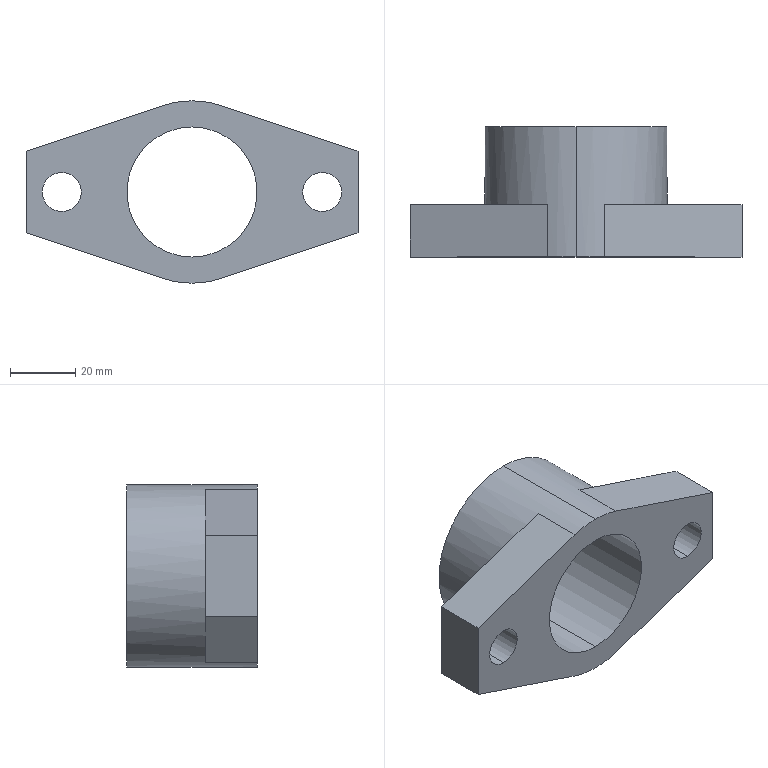Part | SolidWorks | features ICE 3, Extrusion 1, MirrorPattern 1 | 1 solid | 18 faces | box 102 x 40 x 56 mm | volume 73509 mm3 | plane 10 | cylinder 8 | commonest cylinder face diameters 12 x4 40 x2 56 x2
STEP:
#1=CARTESIAN_POINT('',(40.,0.,-6.));
#2=VERTEX_POINT('',#1);
#3=CARTESIAN_POINT('',(40.,0.,6.));
#4=VERTEX_POINT('',#3);
#5=CARTESIAN_POINT('',(40.,0.,0.));
#6=DIRECTION('',(0.,1.,0.));
#7=DIRECTION('',(0.,0.,1.));
#8=AXIS2_PLACEMENT_3D('',#5,#6,#7);
#9=CIRCLE('',#8,6.);
#10=EDGE_CURVE('',#2,#4,#9,.T.);
#11=ORIENTED_EDGE('',*,*,#10,.F.);
#12=CARTESIAN_POINT('',(40.,16.,-6.));
#13=VERTEX_POINT('',#12);
#14=CARTESIAN_POINT('',(40.,0.,-6.));
#15=DIRECTION('',(0.,1.,0.));
#16=VECTOR('',#15,1000.);
#17=LINE('',#14,#16);
#18=EDGE_CURVE('',#2,#13,#17,.T.);
#19=ORIENTED_EDGE('',*,*,#18,.T.);
#20=CARTESIAN_POINT('',(40.,16.,6.));
#21=VERTEX_POINT('',#20);
#22=CARTESIAN_POINT('',(40.,16.,0.));
#23=DIRECTION('',(0.,1.,0.));
#24=DIRECTION('',(0.,0.,1.));
#25=AXIS2_PLACEMENT_3D('',#22,#23,#24);
#26=CIRCLE('',#25,6.);
#27=EDGE_CURVE('',#13,#21,#26,.T.);
#28=ORIENTED_EDGE('',*,*,#27,.T.);
#29=CARTESIAN_POINT('',(40.,0.,6.));
#30=DIRECTION('',(0.,1.,0.));
#31=VECTOR('',#30,1000.);
#32=LINE('',#29,#31);
#33=EDGE_CURVE('',#4,#21,#32,.T.);
#34=ORIENTED_EDGE('',*,*,#33,.F.);
#35=EDGE_LOOP('',(#11,#19,#28,#34));
#36=FACE_OUTER_BOUND('',#35,.T.);
#37=CARTESIAN_POINT('',(40.,0.,0.));
#38=DIRECTION('',(0.,1.,0.));
#39=DIRECTION('',(0.,0.,1.));
#40=AXIS2_PLACEMENT_3D('',#37,#38,#39);
#41=CYLINDRICAL_SURFACE('',#40,6.);
#42=ADVANCED_FACE('',(#36),#41,.F.);
#43=CARTESIAN_POINT('',(-40.,0.,-6.));
#44=VERTEX_POINT('',#43);
#45=CARTESIAN_POINT('',(-40.,0.,6.));
#46=VERTEX_POINT('',#45);
#47=CARTESIAN_POINT('',(-40.,0.,0.));
#48=DIRECTION('',(0.,1.,0.));
#49=DIRECTION('',(0.,0.,1.));
#50=AXIS2_PLACEMENT_3D('',#47,#48,#49);
#51=CIRCLE('',#50,6.);
#52=EDGE_CURVE('',#44,#46,#51,.T.);
#53=ORIENTED_EDGE('',*,*,#52,.F.);
#54=CARTESIAN_POINT('',(-40.,16.,-6.));
#55=VERTEX_POINT('',#54);
#56=CARTESIAN_POINT('',(-40.,0.,-6.));
#57=DIRECTION('',(0.,1.,0.));
#58=VECTOR('',#57,1000.);
#59=LINE('',#56,#58);
#60=EDGE_CURVE('',#44,#55,#59,.T.);
#61=ORIENTED_EDGE('',*,*,#60,.T.);
#62=CARTESIAN_POINT('',(-40.,16.,6.));
#63=VERTEX_POINT('',#62);
#64=CARTESIAN_POINT('',(-40.,16.,0.));
#65=DIRECTION('',(0.,1.,0.));
#66=DIRECTION('',(0.,0.,1.));
#67=AXIS2_PLACEMENT_3D('',#64,#65,#66);
#68=CIRCLE('',#67,6.);
#69=EDGE_CURVE('',#55,#63,#68,.T.);
#70=ORIENTED_EDGE('',*,*,#69,.T.);
#71=CARTESIAN_POINT('',(-40.,0.,6.));
#72=DIRECTION('',(0.,1.,0.));
#73=VECTOR('',#72,1000.);
#74=LINE('',#71,#73);
#75=EDGE_CURVE('',#46,#63,#74,.T.);
#76=ORIENTED_EDGE('',*,*,#75,.F.);
#77=EDGE_LOOP('',(#53,#61,#70,#76));
#78=FACE_OUTER_BOUND('',#77,.T.);
#79=CARTESIAN_POINT('',(-40.,0.,0.));
#80=DIRECTION('',(0.,1.,0.));
#81=DIRECTION('',(0.,0.,1.));
#82=AXIS2_PLACEMENT_3D('',#79,#80,#81);
#83=CYLINDRICAL_SURFACE('',#82,6.);
#84=ADVANCED_FACE('',(#78),#83,.F.);
#85=CARTESIAN_POINT('',(0.,0.,-20.));
#86=VERTEX_POINT('',#85);
#87=CARTESIAN_POINT('',(0.,0.,20.));
#88=VERTEX_POINT('',#87);
#89=CARTESIAN_POINT('',(0.,0.,0.));
#90=DIRECTION('',(0.,1.,0.));
#91=DIRECTION('',(0.,0.,1.));
#92=AXIS2_PLACEMENT_3D('',#89,#90,#91);
#93=CIRCLE('',#92,20.);
#94=EDGE_CURVE('',#86,#88,#93,.T.);
#95=ORIENTED_EDGE('',*,*,#94,.F.);
#96=CARTESIAN_POINT('',(0.,40.,-20.));
#97=VERTEX_POINT('',#96);
#98=CARTESIAN_POINT('',(0.,0.,-20.));
#99=DIRECTION('',(0.,1.,0.));
#100=VECTOR('',#99,1000.);
#101=LINE('',#98,#100);
#102=EDGE_CURVE('',#86,#97,#101,.T.);
#103=ORIENTED_EDGE('',*,*,#102,.T.);
#104=CARTESIAN_POINT('',(0.,40.,20.));
#105=VERTEX_POINT('',#104);
#106=CARTESIAN_POINT('',(0.,40.,0.));
#107=DIRECTION('',(0.,1.,0.));
#108=DIRECTION('',(0.,0.,1.));
#109=AXIS2_PLACEMENT_3D('',#106,#107,#108);
#110=CIRCLE('',#109,20.);
#111=EDGE_CURVE('',#97,#105,#110,.T.);
#112=ORIENTED_EDGE('',*,*,#111,.T.);
#113=CARTESIAN_POINT('',(0.,0.,20.));
#114=DIRECTION('',(0.,1.,0.));
#115=VECTOR('',#114,1000.);
#116=LINE('',#113,#115);
#117=EDGE_CURVE('',#88,#105,#116,.T.);
#118=ORIENTED_EDGE('',*,*,#117,.F.);
#119=EDGE_LOOP('',(#95,#103,#112,#118));
#120=FACE_OUTER_BOUND('',#119,.T.);
#121=CARTESIAN_POINT('',(0.,0.,0.));
#122=DIRECTION('',(0.,1.,0.));
#123=DIRECTION('',(0.,0.,1.));
#124=AXIS2_PLACEMENT_3D('',#121,#122,#123);
#125=CYLINDRICAL_SURFACE('',#124,20.);
#126=ADVANCED_FACE('',(#120),#125,.F.);
#127=CARTESIAN_POINT('',(0.,40.,28.));
#128=VERTEX_POINT('',#127);
#129=CARTESIAN_POINT('',(0.,40.,-28.));
#130=VERTEX_POINT('',#129);
#131=CARTESIAN_POINT('',(0.,40.,0.));
#132=DIRECTION('',(0.,1.,0.));
#133=DIRECTION('',(0.,0.,1.));
#134=AXIS2_PLACEMENT_3D('',#131,#132,#133);
#135=CIRCLE('',#134,28.);
#136=EDGE_CURVE('',#128,#130,#135,.T.);
#137=ORIENTED_EDGE('',*,*,#136,.F.);
#138=CARTESIAN_POINT('',(0.,0.,28.));
#139=VERTEX_POINT('',#138);
#140=CARTESIAN_POINT('',(0.,40.,28.));
#141=DIRECTION('',(0.,-1.,0.));
#142=VECTOR('',#141,1000.);
#143=LINE('',#140,#142);
#144=EDGE_CURVE('',#128,#139,#143,.T.);
#145=ORIENTED_EDGE('',*,*,#144,.T.);
#146=CARTESIAN_POINT('',(8.863,0.,26.56));
#147=VERTEX_POINT('',#146);
#148=CARTESIAN_POINT('',(0.,0.,0.));
#149=DIRECTION('',(0.,1.,0.));
#150=DIRECTION('',(0.,0.,1.));
#151=AXIS2_PLACEMENT_3D('',#148,#149,#150);
#152=CIRCLE('',#151,28.);
#153=EDGE_CURVE('',#139,#147,#152,.T.);
#154=ORIENTED_EDGE('',*,*,#153,.T.);
#155=CARTESIAN_POINT('',(8.863,16.,26.56));
#156=VERTEX_POINT('',#155);
#157=CARTESIAN_POINT('',(8.863,16.,26.56));
#158=DIRECTION('',(0.,-1.,0.));
#159=VECTOR('',#158,1000.);
#160=LINE('',#157,#159);
#161=EDGE_CURVE('',#156,#147,#160,.T.);
#162=ORIENTED_EDGE('',*,*,#161,.F.);
#163=CARTESIAN_POINT('',(8.863,16.,-26.56));
#164=VERTEX_POINT('',#163);
#165=CARTESIAN_POINT('',(0.,16.,0.));
#166=DIRECTION('',(0.,-1.,0.));
#167=DIRECTION('',(0.,0.,-1.));
#168=AXIS2_PLACEMENT_3D('',#165,#166,#167);
#169=CIRCLE('',#168,28.);
#170=EDGE_CURVE('',#164,#156,#169,.T.);
#171=ORIENTED_EDGE('',*,*,#170,.F.);
#172=CARTESIAN_POINT('',(8.863,0.,-26.56));
#173=VERTEX_POINT('',#172);
#174=CARTESIAN_POINT('',(8.863,16.,-26.56));
#175=DIRECTION('',(0.,-1.,0.));
#176=VECTOR('',#175,1000.);
#177=LINE('',#174,#176);
#178=EDGE_CURVE('',#164,#173,#177,.T.);
#179=ORIENTED_EDGE('',*,*,#178,.T.);
#180=CARTESIAN_POINT('',(0.,0.,-28.));
#181=VERTEX_POINT('',#180);
#182=CARTESIAN_POINT('',(0.,0.,0.));
#183=DIRECTION('',(0.,1.,0.));
#184=DIRECTION('',(0.,0.,1.));
#185=AXIS2_PLACEMENT_3D('',#182,#183,#184);
#186=CIRCLE('',#185,28.);
#187=EDGE_CURVE('',#173,#181,#186,.T.);
#188=ORIENTED_EDGE('',*,*,#187,.T.);
#189=CARTESIAN_POINT('',(0.,40.,-28.));
#190=DIRECTION('',(0.,-1.,0.));
#191=VECTOR('',#190,1000.);
#192=LINE('',#189,#191);
#193=EDGE_CURVE('',#130,#181,#192,.T.);
#194=ORIENTED_EDGE('',*,*,#193,.F.);
#195=EDGE_LOOP('',(#137,#145,#154,#162,#171,#179,#188,#194));
#196=FACE_OUTER_BOUND('',#195,.T.);
#197=CARTESIAN_POINT('',(0.,40.,0.));
#198=DIRECTION('',(0.,-1.,0.));
#199=DIRECTION('',(0.,0.,-1.));
#200=AXIS2_PLACEMENT_3D('',#197,#198,#199);
#201=CYLINDRICAL_SURFACE('',#200,28.);
#202=ADVANCED_FACE('',(#196),#201,.T.);
#203=ORIENTED_EDGE('',*,*,#144,.F.);
#204=CARTESIAN_POINT('',(0.,40.,0.));
#205=DIRECTION('',(0.,1.,0.));
#206=DIRECTION('',(0.,0.,1.));
#207=AXIS2_PLACEMENT_3D('',#204,#205,#206);
#208=CIRCLE('',#207,28.);
#209=EDGE_CURVE('',#130,#128,#208,.T.);
#210=ORIENTED_EDGE('',*,*,#209,.F.);
#211=ORIENTED_EDGE('',*,*,#193,.T.);
#212=CARTESIAN_POINT('',(-8.863,0.,-26.56));
#213=VERTEX_POINT('',#212);
#214=CARTESIAN_POINT('',(0.,0.,0.));
#215=DIRECTION('',(0.,1.,0.));
#216=DIRECTION('',(0.,0.,1.));
#217=AXIS2_PLACEMENT_3D('',#214,#215,#216);
#218=CIRCLE('',#217,28.);
#219=EDGE_CURVE('',#181,#213,#218,.T.);
#220=ORIENTED_EDGE('',*,*,#219,.T.);
#221=CARTESIAN_POINT('',(-8.863,16.,-26.56));
#222=VERTEX_POINT('',#221);
#223=CARTESIAN_POINT('',(-8.863,16.,-26.56));
#224=DIRECTION('',(0.,-1.,0.));
#225=VECTOR('',#224,1000.);
#226=LINE('',#223,#225);
#227=EDGE_CURVE('',#222,#213,#226,.T.);
#228=ORIENTED_EDGE('',*,*,#227,.F.);
#229=CARTESIAN_POINT('',(-8.863,16.,26.56));
#230=VERTEX_POINT('',#229);
#231=CARTESIAN_POINT('',(0.,16.,0.));
#232=DIRECTION('',(0.,-1.,0.));
#233=DIRECTION('',(0.,0.,-1.));
#234=AXIS2_PLACEMENT_3D('',#231,#232,#233);
#235=CIRCLE('',#234,28.);
#236=EDGE_CURVE('',#230,#222,#235,.T.);
#237=ORIENTED_EDGE('',*,*,#236,.F.);
#238=CARTESIAN_POINT('',(-8.863,0.,26.56));
#239=VERTEX_POINT('',#238);
#240=CARTESIAN_POINT('',(-8.863,16.,26.56));
#241=DIRECTION('',(0.,-1.,0.));
#242=VECTOR('',#241,1000.);
#243=LINE('',#240,#242);
#244=EDGE_CURVE('',#230,#239,#243,.T.);
#245=ORIENTED_EDGE('',*,*,#244,.T.);
#246=CARTESIAN_POINT('',(0.,0.,0.));
#247=DIRECTION('',(0.,1.,0.));
#248=DIRECTION('',(0.,0.,1.));
#249=AXIS2_PLACEMENT_3D('',#246,#247,#248);
#250=CIRCLE('',#249,28.);
#251=EDGE_CURVE('',#239,#139,#250,.T.);
#252=ORIENTED_EDGE('',*,*,#251,.T.);
#253=EDGE_LOOP('',(#203,#210,#211,#220,#228,#237,#245,#252));
#254=FACE_OUTER_BOUND('',#253,.T.);
#255=CARTESIAN_POINT('',(0.,40.,0.));
#256=DIRECTION('',(0.,-1.,0.));
#257=DIRECTION('',(0.,0.,-1.));
#258=AXIS2_PLACEMENT_3D('',#255,#256,#257);
#259=CYLINDRICAL_SURFACE('',#258,28.);
#260=ADVANCED_FACE('',(#254),#259,.T.);
#261=CARTESIAN_POINT('',(0.,40.,0.));
#262=DIRECTION('',(0.,1.,0.));
#263=DIRECTION('',(0.,0.,1.));
#264=AXIS2_PLACEMENT_3D('',#261,#262,#263);
#265=CIRCLE('',#264,20.);
#266=EDGE_CURVE('',#105,#97,#265,.T.);
#267=ORIENTED_EDGE('',*,*,#266,.F.);
#268=ORIENTED_EDGE('',*,*,#111,.F.);
#269=EDGE_LOOP('',(#267,#268));
#270=FACE_BOUND('',#269,.T.);
#271=ORIENTED_EDGE('',*,*,#209,.T.);
#272=ORIENTED_EDGE('',*,*,#136,.T.);
#273=EDGE_LOOP('',(#271,#272));
#274=FACE_OUTER_BOUND('',#273,.T.);
#275=CARTESIAN_POINT('',(0.,40.,0.));
#276=DIRECTION('',(0.,1.,0.));
#277=DIRECTION('',(0.,0.,1.));
#278=AXIS2_PLACEMENT_3D('',#275,#276,#277);
#279=PLANE('',#278);
#280=ADVANCED_FACE('',(#270,#274),#279,.T.);
#281=CARTESIAN_POINT('',(40.,0.,0.));
#282=DIRECTION('',(0.,1.,0.));
#283=DIRECTION('',(0.,0.,1.));
#284=AXIS2_PLACEMENT_3D('',#281,#282,#283);
#285=CIRCLE('',#284,6.);
#286=EDGE_CURVE('',#4,#2,#285,.T.);
#287=ORIENTED_EDGE('',*,*,#286,.T.);
#288=ORIENTED_EDGE('',*,*,#10,.T.);
#289=EDGE_LOOP('',(#287,#288));
#290=FACE_BOUND('',#289,.T.);
#291=CARTESIAN_POINT('',(-40.,0.,0.));
#292=DIRECTION('',(0.,1.,0.));
#293=DIRECTION('',(0.,0.,1.));
#294=AXIS2_PLACEMENT_3D('',#291,#292,#293);
#295=CIRCLE('',#294,6.);
#296=EDGE_CURVE('',#46,#44,#295,.T.);
#297=ORIENTED_EDGE('',*,*,#296,.T.);
#298=ORIENTED_EDGE('',*,*,#52,.T.);
#299=EDGE_LOOP('',(#297,#298));
#300=FACE_BOUND('',#299,.T.);
#301=CARTESIAN_POINT('',(0.,0.,0.));
#302=DIRECTION('',(0.,1.,0.));
#303=DIRECTION('',(0.,0.,1.));
#304=AXIS2_PLACEMENT_3D('',#301,#302,#303);
#305=CIRCLE('',#304,20.);
#306=EDGE_CURVE('',#88,#86,#305,.T.);
#307=ORIENTED_EDGE('',*,*,#306,.T.);
#308=ORIENTED_EDGE('',*,*,#94,.T.);
#309=EDGE_LOOP('',(#307,#308));
#310=FACE_BOUND('',#309,.T.);
#311=ORIENTED_EDGE('',*,*,#187,.F.);
#312=CARTESIAN_POINT('',(51.,0.,-12.5));
#313=VERTEX_POINT('',#312);
#314=CARTESIAN_POINT('',(51.,0.,-12.5));
#315=DIRECTION('',(-0.9486,0.,-0.3165));
#316=VECTOR('',#315,1000.);
#317=LINE('',#314,#316);
#318=EDGE_CURVE('',#313,#173,#317,.T.);
#319=ORIENTED_EDGE('',*,*,#318,.F.);
#320=CARTESIAN_POINT('',(51.,0.,12.5));
#321=VERTEX_POINT('',#320);
#322=CARTESIAN_POINT('',(51.,0.,-12.5));
#323=DIRECTION('',(0.,0.,-1.));
#324=VECTOR('',#323,1000.);
#325=LINE('',#322,#324);
#326=EDGE_CURVE('',#321,#313,#325,.T.);
#327=ORIENTED_EDGE('',*,*,#326,.F.);
#328=CARTESIAN_POINT('',(51.,0.,12.5));
#329=DIRECTION('',(0.9486,0.,-0.3165));
#330=VECTOR('',#329,1000.);
#331=LINE('',#328,#330);
#332=EDGE_CURVE('',#147,#321,#331,.T.);
#333=ORIENTED_EDGE('',*,*,#332,.F.);
#334=ORIENTED_EDGE('',*,*,#153,.F.);
#335=ORIENTED_EDGE('',*,*,#251,.F.);
#336=CARTESIAN_POINT('',(-51.,0.,12.5));
#337=VERTEX_POINT('',#336);
#338=CARTESIAN_POINT('',(-51.,0.,12.5));
#339=DIRECTION('',(-0.9486,0.,-0.3165));
#340=VECTOR('',#339,1000.);
#341=LINE('',#338,#340);
#342=EDGE_CURVE('',#239,#337,#341,.T.);
#343=ORIENTED_EDGE('',*,*,#342,.T.);
#344=CARTESIAN_POINT('',(-51.,0.,-12.5));
#345=VERTEX_POINT('',#344);
#346=CARTESIAN_POINT('',(-51.,0.,-12.5));
#347=DIRECTION('',(0.,0.,-1.));
#348=VECTOR('',#347,1000.);
#349=LINE('',#346,#348);
#350=EDGE_CURVE('',#337,#345,#349,.T.);
#351=ORIENTED_EDGE('',*,*,#350,.T.);
#352=CARTESIAN_POINT('',(-51.,0.,-12.5));
#353=DIRECTION('',(0.9486,0.,-0.3165));
#354=VECTOR('',#353,1000.);
#355=LINE('',#352,#354);
#356=EDGE_CURVE('',#345,#213,#355,.T.);
#357=ORIENTED_EDGE('',*,*,#356,.T.);
#358=ORIENTED_EDGE('',*,*,#219,.F.);
#359=EDGE_LOOP('',(#311,#319,#327,#333,#334,#335,#343,#351,#357,#358));
#360=FACE_OUTER_BOUND('',#359,.T.);
#361=CARTESIAN_POINT('',(0.,0.,0.));
#362=DIRECTION('',(0.,1.,0.));
#363=DIRECTION('',(0.,0.,1.));
#364=AXIS2_PLACEMENT_3D('',#361,#362,#363);
#365=PLANE('',#364);
#366=ADVANCED_FACE('',(#290,#300,#310,#360),#365,.F.);
#367=CARTESIAN_POINT('',(-40.,16.,0.));
#368=DIRECTION('',(0.,1.,0.));
#369=DIRECTION('',(0.,0.,1.));
#370=AXIS2_PLACEMENT_3D('',#367,#368,#369);
#371=CIRCLE('',#370,6.);
#372=EDGE_CURVE('',#63,#55,#371,.T.);
#373=ORIENTED_EDGE('',*,*,#372,.F.);
#374=ORIENTED_EDGE('',*,*,#69,.F.);
#375=EDGE_LOOP('',(#373,#374));
#376=FACE_BOUND('',#375,.T.);
#377=CARTESIAN_POINT('',(-51.,16.,12.5));
#378=VERTEX_POINT('',#377);
#379=CARTESIAN_POINT('',(-51.,16.,12.5));
#380=DIRECTION('',(-0.9486,0.,-0.3165));
#381=VECTOR('',#380,1000.);
#382=LINE('',#379,#381);
#383=EDGE_CURVE('',#230,#378,#382,.T.);
#384=ORIENTED_EDGE('',*,*,#383,.F.);
#385=ORIENTED_EDGE('',*,*,#236,.T.);
#386=CARTESIAN_POINT('',(-51.,16.,-12.5));
#387=VERTEX_POINT('',#386);
#388=CARTESIAN_POINT('',(-51.,16.,-12.5));
#389=DIRECTION('',(0.9486,0.,-0.3165));
#390=VECTOR('',#389,1000.);
#391=LINE('',#388,#390);
#392=EDGE_CURVE('',#387,#222,#391,.T.);
#393=ORIENTED_EDGE('',*,*,#392,.F.);
#394=CARTESIAN_POINT('',(-51.,16.,-12.5));
#395=DIRECTION('',(0.,0.,-1.));
#396=VECTOR('',#395,1000.);
#397=LINE('',#394,#396);
#398=EDGE_CURVE('',#378,#387,#397,.T.);
#399=ORIENTED_EDGE('',*,*,#398,.F.);
#400=EDGE_LOOP('',(#384,#385,#393,#399));
#401=FACE_OUTER_BOUND('',#400,.T.);
#402=CARTESIAN_POINT('',(0.,16.,0.));
#403=DIRECTION('',(0.,-1.,0.));
#404=DIRECTION('',(0.,0.,-1.));
#405=AXIS2_PLACEMENT_3D('',#402,#403,#404);
#406=PLANE('',#405);
#407=ADVANCED_FACE('',(#376,#401),#406,.F.);
#408=ORIENTED_EDGE('',*,*,#356,.F.);
#409=CARTESIAN_POINT('',(-51.,16.,-12.5));
#410=DIRECTION('',(0.,-1.,0.));
#411=VECTOR('',#410,1000.);
#412=LINE('',#409,#411);
#413=EDGE_CURVE('',#387,#345,#412,.T.);
#414=ORIENTED_EDGE('',*,*,#413,.F.);
#415=ORIENTED_EDGE('',*,*,#392,.T.);
#416=ORIENTED_EDGE('',*,*,#227,.T.);
#417=EDGE_LOOP('',(#408,#414,#415,#416));
#418=FACE_OUTER_BOUND('',#417,.T.);
#419=CARTESIAN_POINT('',(-51.,16.,-12.5));
#420=DIRECTION('',(-0.3165,0.,-0.9486));
#421=DIRECTION('',(-0.9486,0.,0.3165));
#422=AXIS2_PLACEMENT_3D('',#419,#420,#421);
#423=PLANE('',#422);
#424=ADVANCED_FACE('',(#418),#423,.T.);
#425=ORIENTED_EDGE('',*,*,#350,.F.);
#426=CARTESIAN_POINT('',(-51.,16.,12.5));
#427=DIRECTION('',(0.,-1.,0.));
#428=VECTOR('',#427,1000.);
#429=LINE('',#426,#428);
#430=EDGE_CURVE('',#378,#337,#429,.T.);
#431=ORIENTED_EDGE('',*,*,#430,.F.);
#432=ORIENTED_EDGE('',*,*,#398,.T.);
#433=ORIENTED_EDGE('',*,*,#413,.T.);
#434=EDGE_LOOP('',(#425,#431,#432,#433));
#435=FACE_OUTER_BOUND('',#434,.T.);
#436=CARTESIAN_POINT('',(-51.,16.,-12.5));
#437=DIRECTION('',(-1.,0.,0.));
#438=DIRECTION('',(0.,0.,1.));
#439=AXIS2_PLACEMENT_3D('',#436,#437,#438);
#440=PLANE('',#439);
#441=ADVANCED_FACE('',(#435),#440,.T.);
#442=ORIENTED_EDGE('',*,*,#342,.F.);
#443=ORIENTED_EDGE('',*,*,#244,.F.);
#444=ORIENTED_EDGE('',*,*,#383,.T.);
#445=ORIENTED_EDGE('',*,*,#430,.T.);
#446=EDGE_LOOP('',(#442,#443,#444,#445));
#447=FACE_OUTER_BOUND('',#446,.T.);
#448=CARTESIAN_POINT('',(-51.,16.,12.5));
#449=DIRECTION('',(-0.3165,0.,0.9486));
#450=DIRECTION('',(0.9486,0.,0.3165));
#451=AXIS2_PLACEMENT_3D('',#448,#449,#450);
#452=PLANE('',#451);
#453=ADVANCED_FACE('',(#447),#452,.T.);
#454=CARTESIAN_POINT('',(40.,16.,0.));
#455=DIRECTION('',(0.,1.,0.));
#456=DIRECTION('',(0.,0.,1.));
#457=AXIS2_PLACEMENT_3D('',#454,#455,#456);
#458=CIRCLE('',#457,6.);
#459=EDGE_CURVE('',#21,#13,#458,.T.);
#460=ORIENTED_EDGE('',*,*,#459,.F.);
#461=ORIENTED_EDGE('',*,*,#27,.F.);
#462=EDGE_LOOP('',(#460,#461));
#463=FACE_BOUND('',#462,.T.);
#464=CARTESIAN_POINT('',(51.,16.,-12.5));
#465=VERTEX_POINT('',#464);
#466=CARTESIAN_POINT('',(51.,16.,-12.5));
#467=DIRECTION('',(-0.9486,0.,-0.3165));
#468=VECTOR('',#467,1000.);
#469=LINE('',#466,#468);
#470=EDGE_CURVE('',#465,#164,#469,.T.);
#471=ORIENTED_EDGE('',*,*,#470,.T.);
#472=ORIENTED_EDGE('',*,*,#170,.T.);
#473=CARTESIAN_POINT('',(51.,16.,12.5));
#474=VERTEX_POINT('',#473);
#475=CARTESIAN_POINT('',(51.,16.,12.5));
#476=DIRECTION('',(0.9486,0.,-0.3165));
#477=VECTOR('',#476,1000.);
#478=LINE('',#475,#477);
#479=EDGE_CURVE('',#156,#474,#478,.T.);
#480=ORIENTED_EDGE('',*,*,#479,.T.);
#481=CARTESIAN_POINT('',(51.,16.,-12.5));
#482=DIRECTION('',(0.,0.,-1.));
#483=VECTOR('',#482,1000.);
#484=LINE('',#481,#483);
#485=EDGE_CURVE('',#474,#465,#484,.T.);
#486=ORIENTED_EDGE('',*,*,#485,.T.);
#487=EDGE_LOOP('',(#471,#472,#480,#486));
#488=FACE_OUTER_BOUND('',#487,.T.);
#489=CARTESIAN_POINT('',(0.,16.,0.));
#490=DIRECTION('',(0.,-1.,0.));
#491=DIRECTION('',(0.,0.,-1.));
#492=AXIS2_PLACEMENT_3D('',#489,#490,#491);
#493=PLANE('',#492);
#494=ADVANCED_FACE('',(#463,#488),#493,.F.);
#495=ORIENTED_EDGE('',*,*,#332,.T.);
#496=CARTESIAN_POINT('',(51.,16.,12.5));
#497=DIRECTION('',(0.,-1.,0.));
#498=VECTOR('',#497,1000.);
#499=LINE('',#496,#498);
#500=EDGE_CURVE('',#474,#321,#499,.T.);
#501=ORIENTED_EDGE('',*,*,#500,.F.);
#502=ORIENTED_EDGE('',*,*,#479,.F.);
#503=ORIENTED_EDGE('',*,*,#161,.T.);
#504=EDGE_LOOP('',(#495,#501,#502,#503));
#505=FACE_OUTER_BOUND('',#504,.T.);
#506=CARTESIAN_POINT('',(51.,16.,12.5));
#507=DIRECTION('',(-0.3165,0.,-0.9486));
#508=DIRECTION('',(-0.9486,0.,0.3165));
#509=AXIS2_PLACEMENT_3D('',#506,#507,#508);
#510=PLANE('',#509);
#511=ADVANCED_FACE('',(#505),#510,.F.);
#512=ORIENTED_EDGE('',*,*,#326,.T.);
#513=CARTESIAN_POINT('',(51.,16.,-12.5));
#514=DIRECTION('',(0.,-1.,0.));
#515=VECTOR('',#514,1000.);
#516=LINE('',#513,#515);
#517=EDGE_CURVE('',#465,#313,#516,.T.);
#518=ORIENTED_EDGE('',*,*,#517,.F.);
#519=ORIENTED_EDGE('',*,*,#485,.F.);
#520=ORIENTED_EDGE('',*,*,#500,.T.);
#521=EDGE_LOOP('',(#512,#518,#519,#520));
#522=FACE_OUTER_BOUND('',#521,.T.);
#523=CARTESIAN_POINT('',(51.,16.,-12.5));
#524=DIRECTION('',(-1.,0.,0.));
#525=DIRECTION('',(0.,0.,1.));
#526=AXIS2_PLACEMENT_3D('',#523,#524,#525);
#527=PLANE('',#526);
#528=ADVANCED_FACE('',(#522),#527,.F.);
#529=ORIENTED_EDGE('',*,*,#318,.T.);
#530=ORIENTED_EDGE('',*,*,#178,.F.);
#531=ORIENTED_EDGE('',*,*,#470,.F.);
#532=ORIENTED_EDGE('',*,*,#517,.T.);
#533=EDGE_LOOP('',(#529,#530,#531,#532));
#534=FACE_OUTER_BOUND('',#533,.T.);
#535=CARTESIAN_POINT('',(51.,16.,-12.5));
#536=DIRECTION('',(-0.3165,0.,0.9486));
#537=DIRECTION('',(0.9486,0.,0.3165));
#538=AXIS2_PLACEMENT_3D('',#535,#536,#537);
#539=PLANE('',#538);
#540=ADVANCED_FACE('',(#534),#539,.F.);
#541=ORIENTED_EDGE('',*,*,#102,.F.);
#542=ORIENTED_EDGE('',*,*,#306,.F.);
#543=ORIENTED_EDGE('',*,*,#117,.T.);
#544=ORIENTED_EDGE('',*,*,#266,.T.);
#545=EDGE_LOOP('',(#541,#542,#543,#544));
#546=FACE_OUTER_BOUND('',#545,.T.);
#547=CARTESIAN_POINT('',(0.,0.,0.));
#548=DIRECTION('',(0.,1.,0.));
#549=DIRECTION('',(0.,0.,1.));
#550=AXIS2_PLACEMENT_3D('',#547,#548,#549);
#551=CYLINDRICAL_SURFACE('',#550,20.);
#552=ADVANCED_FACE('',(#546),#551,.F.);
#553=ORIENTED_EDGE('',*,*,#60,.F.);
#554=ORIENTED_EDGE('',*,*,#296,.F.);
#555=ORIENTED_EDGE('',*,*,#75,.T.);
#556=ORIENTED_EDGE('',*,*,#372,.T.);
#557=EDGE_LOOP('',(#553,#554,#555,#556));
#558=FACE_OUTER_BOUND('',#557,.T.);
#559=CARTESIAN_POINT('',(-40.,0.,0.));
#560=DIRECTION('',(0.,1.,0.));
#561=DIRECTION('',(0.,0.,1.));
#562=AXIS2_PLACEMENT_3D('',#559,#560,#561);
#563=CYLINDRICAL_SURFACE('',#562,6.);
#564=ADVANCED_FACE('',(#558),#563,.F.);
#565=ORIENTED_EDGE('',*,*,#18,.F.);
#566=ORIENTED_EDGE('',*,*,#286,.F.);
#567=ORIENTED_EDGE('',*,*,#33,.T.);
#568=ORIENTED_EDGE('',*,*,#459,.T.);
#569=EDGE_LOOP('',(#565,#566,#567,#568));
#570=FACE_OUTER_BOUND('',#569,.T.);
#571=CARTESIAN_POINT('',(40.,0.,0.));
#572=DIRECTION('',(0.,1.,0.));
#573=DIRECTION('',(0.,0.,1.));
#574=AXIS2_PLACEMENT_3D('',#571,#572,#573);
#575=CYLINDRICAL_SURFACE('',#574,6.);
#576=ADVANCED_FACE('',(#570),#575,.F.);
#577=CLOSED_SHELL('',(#42,#84,#126,#202,#260,#280,#366,#407,#424,#441,#453,#494,#511,#528,#540,#552,#564,#576));
#578=MANIFOLD_SOLID_BREP('',#577);
#579=CARTESIAN_POINT('',(0.,0.,0.));
#580=DIRECTION('',(0.,0.,1.));
#581=DIRECTION('',(1.,0.,0.));
#582=AXIS2_PLACEMENT_3D('',#579,#580,#581);
#583=(LENGTH_UNIT()NAMED_UNIT(*)SI_UNIT(.MILLI.,.METRE.));
#584=UNCERTAINTY_MEASURE_WITH_UNIT(LENGTH_MEASURE(0.00001),#583,'','');
#585=(NAMED_UNIT(*)PLANE_ANGLE_UNIT()SI_UNIT($,.RADIAN.));
#586=(NAMED_UNIT(*)SI_UNIT($,.STERADIAN.)SOLID_ANGLE_UNIT());
#587=(GEOMETRIC_REPRESENTATION_CONTEXT(3)GLOBAL_UNCERTAINTY_ASSIGNED_CONTEXT((#584))GLOBAL_UNIT_ASSIGNED_CONTEXT((#583,#585,#586))REPRESENTATION_CONTEXT('',''));
#588=ADVANCED_BREP_SHAPE_REPRESENTATION('',(#578,#582),#587);